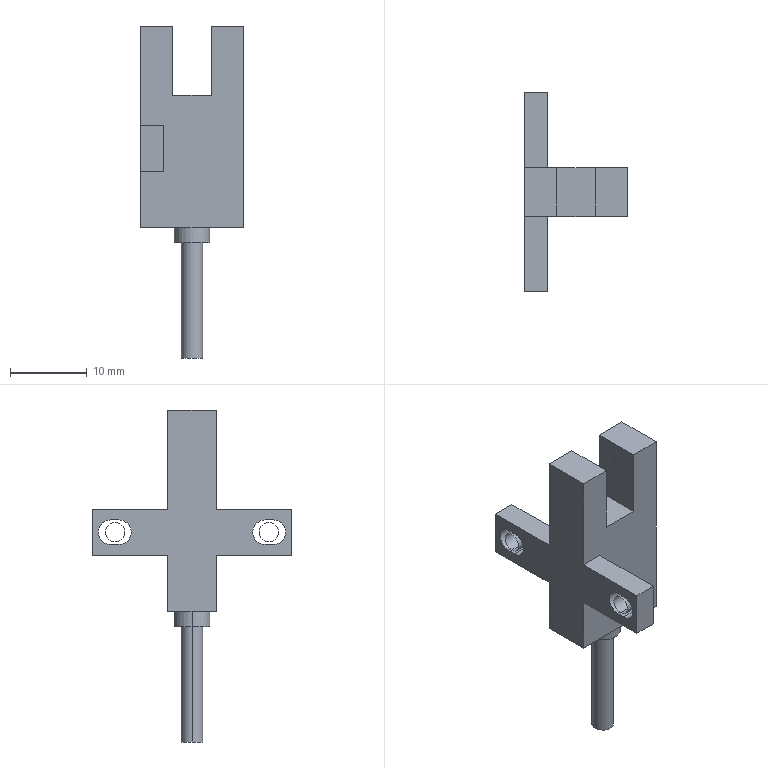Part | NX | features BREP 3 | 1 solid | 51 faces | box 13.4 x 26 x 43.2 mm | volume 2373 mm3 | plane 39 | cylinder 12 | commonest cylinder face diameters 2.5 x4 3.2 x4 2.8 x2 4.6 x2